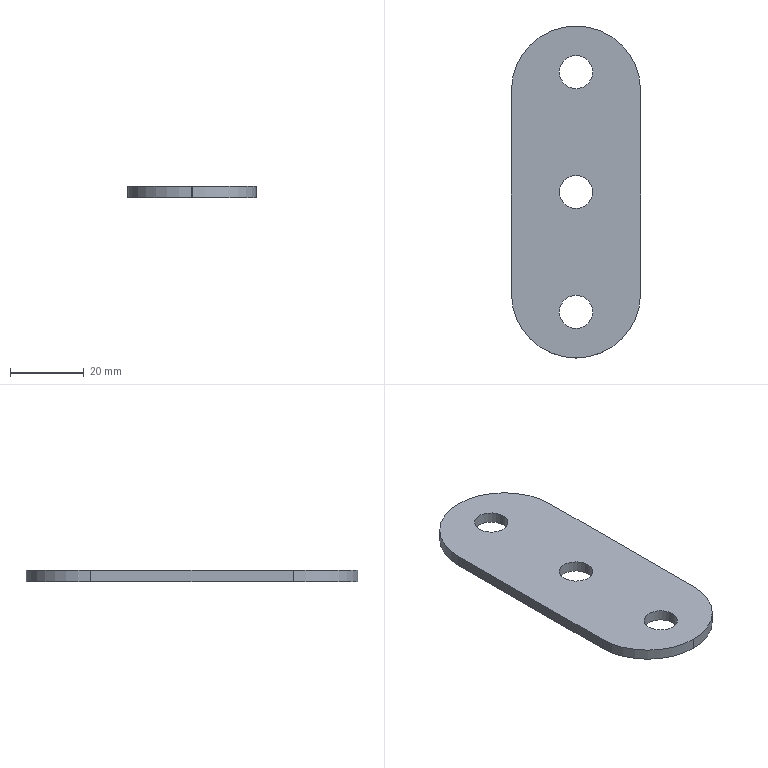Part | STEP file | 5091502 | 1 solid | 13 faces | box 35 x 90 x 3 mm | volume 8089 mm3 | cylinder 7 | plane 6 | commonest cylinder face diameters 34.998 x4 9 x3
STEP:
#1=CARTESIAN_POINT('',(0.,0.,0.));
#2=DIRECTION('',(0.,0.,1.));
#3=DIRECTION('',(1.,0.,0.));
#4=AXIS2_PLACEMENT_3D('',#1,#2,#3);
#5=CARTESIAN_POINT('',(4.5,0.,3.));
#6=VERTEX_POINT('',#5);
#7=CARTESIAN_POINT('',(0.,0.,3.));
#8=DIRECTION('',(0.,0.,1.));
#9=DIRECTION('',(1.,0.,0.));
#10=AXIS2_PLACEMENT_3D('',#7,#8,#9);
#11=CIRCLE('',#10,4.5);
#12=CARTESIAN_POINT('',(0.001,27.501,3.));
#13=DIRECTION('',(0.,0.,-1.));
#14=DIRECTION('',(-1.,0.,0.));
#15=AXIS2_PLACEMENT_3D('',#12,#13,#14);
#16=PLANE('',#15);
#17=CARTESIAN_POINT('',(-4.499,-27.501));
#18=CARTESIAN_POINT('',(-4.499,-19.707));
#19=CARTESIAN_POINT('',(2.251,-23.604));
#20=CARTESIAN_POINT('',(9.001,-27.501));
#21=CARTESIAN_POINT('',(2.251,-31.398));
#22=CARTESIAN_POINT('',(-4.499,-35.295));
#23=CARTESIAN_POINT('',(-4.499,-27.501));
#24=(BOUNDED_CURVE()B_SPLINE_CURVE(2,(#17,#18,#19,#20,#21,#22,#23),.UNSPECIFIED.,.T.,.F.)B_SPLINE_CURVE_WITH_KNOTS((1,2,2,2,2,1),(-2.094,0.,2.094,4.189,6.283,8.378),.UNSPECIFIED.)CURVE()GEOMETRIC_REPRESENTATION_ITEM()RATIONAL_B_SPLINE_CURVE((1.,0.5,1.,0.5,1.,0.5,1.))REPRESENTATION_ITEM(''));
#25=(GEOMETRIC_REPRESENTATION_CONTEXT(2)PARAMETRIC_REPRESENTATION_CONTEXT()REPRESENTATION_CONTEXT('',''));
#26=DEFINITIONAL_REPRESENTATION('',(#24),#25);
#27=PCURVE('',#16,#26);
#28=CARTESIAN_POINT('',(0.,0.,3.));
#29=DIRECTION('',(0.,0.,-1.));
#30=DIRECTION('',(-1.,0.,0.));
#31=AXIS2_PLACEMENT_3D('',#28,#29,#30);
#32=CYLINDRICAL_SURFACE('',#31,4.5);
#33=CARTESIAN_POINT('',(9.425,0.));
#34=DIRECTION('',(-1.,0.));
#35=VECTOR('',#34,1.);
#36=LINE('',#33,#35);
#37=(GEOMETRIC_REPRESENTATION_CONTEXT(2)PARAMETRIC_REPRESENTATION_CONTEXT()REPRESENTATION_CONTEXT('',''));
#38=DEFINITIONAL_REPRESENTATION('',(#36),#37);
#39=PCURVE('',#32,#38);
#40=SURFACE_CURVE('',#11,(#27,#39),.PCURVE_S1.);
#41=EDGE_CURVE('',#6,#6,#40,.T.);
#42=ORIENTED_EDGE('',*,*,#41,.F.);
#43=EDGE_LOOP('',(#42));
#44=FACE_BOUND('',#43,.T.);
#45=CARTESIAN_POINT('',(17.5,27.501,3.));
#46=VERTEX_POINT('',#45);
#47=CARTESIAN_POINT('',(0.001,45.,3.));
#48=VERTEX_POINT('',#47);
#49=CARTESIAN_POINT('',(0.001,27.501,3.));
#50=DIRECTION('',(0.,0.,1.));
#51=DIRECTION('',(-1.,0.,0.));
#52=AXIS2_PLACEMENT_3D('',#49,#50,#51);
#53=CIRCLE('',#52,17.499);
#54=CARTESIAN_POINT('',(17.499,0.));
#55=CARTESIAN_POINT('',(17.499,-30.309));
#56=CARTESIAN_POINT('',(-8.749,-15.155));
#57=CARTESIAN_POINT('',(-34.998,0.));
#58=CARTESIAN_POINT('',(-8.749,15.155));
#59=CARTESIAN_POINT('',(17.499,30.309));
#60=CARTESIAN_POINT('',(17.499,0.));
#61=(BOUNDED_CURVE()B_SPLINE_CURVE(2,(#54,#55,#56,#57,#58,#59,#60),.UNSPECIFIED.,.T.,.F.)B_SPLINE_CURVE_WITH_KNOTS((1,2,2,2,2,1),(-2.094,0.,2.094,4.189,6.283,8.378),.UNSPECIFIED.)CURVE()GEOMETRIC_REPRESENTATION_ITEM()RATIONAL_B_SPLINE_CURVE((1.,0.5,1.,0.5,1.,0.5,1.))REPRESENTATION_ITEM(''));
#62=(GEOMETRIC_REPRESENTATION_CONTEXT(2)PARAMETRIC_REPRESENTATION_CONTEXT()REPRESENTATION_CONTEXT('',''));
#63=DEFINITIONAL_REPRESENTATION('',(#61),#62);
#64=PCURVE('',#16,#63);
#65=CARTESIAN_POINT('',(0.001,27.501,3.));
#66=DIRECTION('',(0.,0.,-1.));
#67=DIRECTION('',(-1.,0.,0.));
#68=AXIS2_PLACEMENT_3D('',#65,#66,#67);
#69=CYLINDRICAL_SURFACE('',#68,17.499);
#70=CARTESIAN_POINT('',(6.283,0.));
#71=DIRECTION('',(-1.,0.));
#72=VECTOR('',#71,1.);
#73=LINE('',#70,#72);
#74=(GEOMETRIC_REPRESENTATION_CONTEXT(2)PARAMETRIC_REPRESENTATION_CONTEXT()REPRESENTATION_CONTEXT('',''));
#75=DEFINITIONAL_REPRESENTATION('',(#73),#74);
#76=PCURVE('',#69,#75);
#77=SURFACE_CURVE('',#53,(#64,#76),.PCURVE_S1.);
#78=EDGE_CURVE('',#46,#48,#77,.T.);
#79=ORIENTED_EDGE('',*,*,#78,.T.);
#80=CARTESIAN_POINT('',(-0.001,45.,3.));
#81=VERTEX_POINT('',#80);
#82=CARTESIAN_POINT('',(-0.001,45.,3.));
#83=DIRECTION('',(-1.,0.,0.));
#84=VECTOR('',#83,1.);
#85=LINE('',#82,#84);
#86=CARTESIAN_POINT('',(0.002,17.499));
#87=DIRECTION('',(1.,0.));
#88=VECTOR('',#87,1.);
#89=LINE('',#86,#88);
#90=(GEOMETRIC_REPRESENTATION_CONTEXT(2)PARAMETRIC_REPRESENTATION_CONTEXT()REPRESENTATION_CONTEXT('',''));
#91=DEFINITIONAL_REPRESENTATION('',(#89),#90);
#92=PCURVE('',#16,#91);
#93=CARTESIAN_POINT('',(-0.001,45.,3.));
#94=DIRECTION('',(0.,-1.,0.));
#95=DIRECTION('',(0.,0.,-1.));
#96=AXIS2_PLACEMENT_3D('',#93,#94,#95);
#97=PLANE('',#96);
#98=CARTESIAN_POINT('',(0.,0.));
#99=DIRECTION('',(0.,-1.));
#100=VECTOR('',#99,1.);
#101=LINE('',#98,#100);
#102=(GEOMETRIC_REPRESENTATION_CONTEXT(2)PARAMETRIC_REPRESENTATION_CONTEXT()REPRESENTATION_CONTEXT('',''));
#103=DEFINITIONAL_REPRESENTATION('',(#101),#102);
#104=PCURVE('',#97,#103);
#105=SURFACE_CURVE('',#85,(#92,#104),.PCURVE_S1.);
#106=EDGE_CURVE('',#48,#81,#105,.T.);
#107=ORIENTED_EDGE('',*,*,#106,.T.);
#108=CARTESIAN_POINT('',(-17.5,27.501,3.));
#109=VERTEX_POINT('',#108);
#110=CARTESIAN_POINT('',(-0.001,27.501,3.));
#111=DIRECTION('',(0.,0.,1.));
#112=DIRECTION('',(-1.,0.,0.));
#113=AXIS2_PLACEMENT_3D('',#110,#111,#112);
#114=CIRCLE('',#113,17.499);
#115=CARTESIAN_POINT('',(17.501,0.));
#116=CARTESIAN_POINT('',(17.501,-30.309));
#117=CARTESIAN_POINT('',(-8.748,-15.155));
#118=CARTESIAN_POINT('',(-34.996,0.));
#119=CARTESIAN_POINT('',(-8.748,15.155));
#120=CARTESIAN_POINT('',(17.501,30.309));
#121=CARTESIAN_POINT('',(17.501,0.));
#122=(BOUNDED_CURVE()B_SPLINE_CURVE(2,(#115,#116,#117,#118,#119,#120,#121),.UNSPECIFIED.,.T.,.F.)B_SPLINE_CURVE_WITH_KNOTS((1,2,2,2,2,1),(-2.094,0.,2.094,4.189,6.283,8.378),.UNSPECIFIED.)CURVE()GEOMETRIC_REPRESENTATION_ITEM()RATIONAL_B_SPLINE_CURVE((1.,0.5,1.,0.5,1.,0.5,1.))REPRESENTATION_ITEM(''));
#123=(GEOMETRIC_REPRESENTATION_CONTEXT(2)PARAMETRIC_REPRESENTATION_CONTEXT()REPRESENTATION_CONTEXT('',''));
#124=DEFINITIONAL_REPRESENTATION('',(#122),#123);
#125=PCURVE('',#16,#124);
#126=CARTESIAN_POINT('',(-0.001,27.501,3.));
#127=DIRECTION('',(0.,0.,-1.));
#128=DIRECTION('',(-1.,0.,0.));
#129=AXIS2_PLACEMENT_3D('',#126,#127,#128);
#130=CYLINDRICAL_SURFACE('',#129,17.499);
#131=CARTESIAN_POINT('',(6.283,0.));
#132=DIRECTION('',(-1.,0.));
#133=VECTOR('',#132,1.);
#134=LINE('',#131,#133);
#135=(GEOMETRIC_REPRESENTATION_CONTEXT(2)PARAMETRIC_REPRESENTATION_CONTEXT()REPRESENTATION_CONTEXT('',''));
#136=DEFINITIONAL_REPRESENTATION('',(#134),#135);
#137=PCURVE('',#130,#136);
#138=SURFACE_CURVE('',#114,(#125,#137),.PCURVE_S1.);
#139=EDGE_CURVE('',#81,#109,#138,.T.);
#140=ORIENTED_EDGE('',*,*,#139,.T.);
#141=CARTESIAN_POINT('',(-17.5,-27.501,3.));
#142=VERTEX_POINT('',#141);
#143=CARTESIAN_POINT('',(-17.5,27.501,3.));
#144=DIRECTION('',(0.,-1.,0.));
#145=VECTOR('',#144,1.);
#146=LINE('',#143,#145);
#147=CARTESIAN_POINT('',(17.501,0.));
#148=DIRECTION('',(0.,-1.));
#149=VECTOR('',#148,1.);
#150=LINE('',#147,#149);
#151=(GEOMETRIC_REPRESENTATION_CONTEXT(2)PARAMETRIC_REPRESENTATION_CONTEXT()REPRESENTATION_CONTEXT('',''));
#152=DEFINITIONAL_REPRESENTATION('',(#150),#151);
#153=PCURVE('',#16,#152);
#154=CARTESIAN_POINT('',(-17.5,27.501,3.));
#155=DIRECTION('',(1.,0.,0.));
#156=DIRECTION('',(0.,1.,0.));
#157=AXIS2_PLACEMENT_3D('',#154,#155,#156);
#158=PLANE('',#157);
#159=CARTESIAN_POINT('',(0.,0.));
#160=DIRECTION('',(-1.,0.));
#161=VECTOR('',#160,1.);
#162=LINE('',#159,#161);
#163=(GEOMETRIC_REPRESENTATION_CONTEXT(2)PARAMETRIC_REPRESENTATION_CONTEXT()REPRESENTATION_CONTEXT('',''));
#164=DEFINITIONAL_REPRESENTATION('',(#162),#163);
#165=PCURVE('',#158,#164);
#166=SURFACE_CURVE('',#146,(#153,#165),.PCURVE_S1.);
#167=EDGE_CURVE('',#109,#142,#166,.T.);
#168=ORIENTED_EDGE('',*,*,#167,.T.);
#169=CARTESIAN_POINT('',(-0.001,-45.,3.));
#170=VERTEX_POINT('',#169);
#171=CARTESIAN_POINT('',(-0.001,-27.501,3.));
#172=DIRECTION('',(0.,0.,1.));
#173=DIRECTION('',(-1.,0.,0.));
#174=AXIS2_PLACEMENT_3D('',#171,#172,#173);
#175=CIRCLE('',#174,17.499);
#176=CARTESIAN_POINT('',(17.501,-55.002));
#177=CARTESIAN_POINT('',(17.501,-85.311));
#178=CARTESIAN_POINT('',(-8.748,-70.157));
#179=CARTESIAN_POINT('',(-34.996,-55.002));
#180=CARTESIAN_POINT('',(-8.748,-39.847));
#181=CARTESIAN_POINT('',(17.501,-24.693));
#182=CARTESIAN_POINT('',(17.501,-55.002));
#183=(BOUNDED_CURVE()B_SPLINE_CURVE(2,(#176,#177,#178,#179,#180,#181,#182),.UNSPECIFIED.,.T.,.F.)B_SPLINE_CURVE_WITH_KNOTS((1,2,2,2,2,1),(-2.094,0.,2.094,4.189,6.283,8.378),.UNSPECIFIED.)CURVE()GEOMETRIC_REPRESENTATION_ITEM()RATIONAL_B_SPLINE_CURVE((1.,0.5,1.,0.5,1.,0.5,1.))REPRESENTATION_ITEM(''));
#184=(GEOMETRIC_REPRESENTATION_CONTEXT(2)PARAMETRIC_REPRESENTATION_CONTEXT()REPRESENTATION_CONTEXT('',''));
#185=DEFINITIONAL_REPRESENTATION('',(#183),#184);
#186=PCURVE('',#16,#185);
#187=CARTESIAN_POINT('',(-0.001,-27.501,3.));
#188=DIRECTION('',(0.,0.,-1.));
#189=DIRECTION('',(-1.,0.,0.));
#190=AXIS2_PLACEMENT_3D('',#187,#188,#189);
#191=CYLINDRICAL_SURFACE('',#190,17.499);
#192=CARTESIAN_POINT('',(6.283,0.));
#193=DIRECTION('',(-1.,0.));
#194=VECTOR('',#193,1.);
#195=LINE('',#192,#194);
#196=(GEOMETRIC_REPRESENTATION_CONTEXT(2)PARAMETRIC_REPRESENTATION_CONTEXT()REPRESENTATION_CONTEXT('',''));
#197=DEFINITIONAL_REPRESENTATION('',(#195),#196);
#198=PCURVE('',#191,#197);
#199=SURFACE_CURVE('',#175,(#186,#198),.PCURVE_S1.);
#200=EDGE_CURVE('',#142,#170,#199,.T.);
#201=ORIENTED_EDGE('',*,*,#200,.T.);
#202=CARTESIAN_POINT('',(0.001,-45.,3.));
#203=VERTEX_POINT('',#202);
#204=CARTESIAN_POINT('',(-0.001,-45.,3.));
#205=DIRECTION('',(1.,0.,0.));
#206=VECTOR('',#205,1.);
#207=LINE('',#204,#206);
#208=CARTESIAN_POINT('',(0.002,-72.501));
#209=DIRECTION('',(-1.,0.));
#210=VECTOR('',#209,1.);
#211=LINE('',#208,#210);
#212=(GEOMETRIC_REPRESENTATION_CONTEXT(2)PARAMETRIC_REPRESENTATION_CONTEXT()REPRESENTATION_CONTEXT('',''));
#213=DEFINITIONAL_REPRESENTATION('',(#211),#212);
#214=PCURVE('',#16,#213);
#215=CARTESIAN_POINT('',(-0.001,-45.,3.));
#216=DIRECTION('',(0.,1.,0.));
#217=DIRECTION('',(0.,0.,1.));
#218=AXIS2_PLACEMENT_3D('',#215,#216,#217);
#219=PLANE('',#218);
#220=CARTESIAN_POINT('',(0.,0.));
#221=DIRECTION('',(0.,1.));
#222=VECTOR('',#221,1.);
#223=LINE('',#220,#222);
#224=(GEOMETRIC_REPRESENTATION_CONTEXT(2)PARAMETRIC_REPRESENTATION_CONTEXT()REPRESENTATION_CONTEXT('',''));
#225=DEFINITIONAL_REPRESENTATION('',(#223),#224);
#226=PCURVE('',#219,#225);
#227=SURFACE_CURVE('',#207,(#214,#226),.PCURVE_S1.);
#228=EDGE_CURVE('',#170,#203,#227,.T.);
#229=ORIENTED_EDGE('',*,*,#228,.T.);
#230=CARTESIAN_POINT('',(17.5,-27.501,3.));
#231=VERTEX_POINT('',#230);
#232=CARTESIAN_POINT('',(0.001,-27.501,3.));
#233=DIRECTION('',(0.,0.,1.));
#234=DIRECTION('',(-1.,0.,0.));
#235=AXIS2_PLACEMENT_3D('',#232,#233,#234);
#236=CIRCLE('',#235,17.499);
#237=CARTESIAN_POINT('',(17.499,-55.002));
#238=CARTESIAN_POINT('',(17.499,-85.311));
#239=CARTESIAN_POINT('',(-8.749,-70.157));
#240=CARTESIAN_POINT('',(-34.998,-55.002));
#241=CARTESIAN_POINT('',(-8.749,-39.847));
#242=CARTESIAN_POINT('',(17.499,-24.693));
#243=CARTESIAN_POINT('',(17.499,-55.002));
#244=(BOUNDED_CURVE()B_SPLINE_CURVE(2,(#237,#238,#239,#240,#241,#242,#243),.UNSPECIFIED.,.T.,.F.)B_SPLINE_CURVE_WITH_KNOTS((1,2,2,2,2,1),(-2.094,0.,2.094,4.189,6.283,8.378),.UNSPECIFIED.)CURVE()GEOMETRIC_REPRESENTATION_ITEM()RATIONAL_B_SPLINE_CURVE((1.,0.5,1.,0.5,1.,0.5,1.))REPRESENTATION_ITEM(''));
#245=(GEOMETRIC_REPRESENTATION_CONTEXT(2)PARAMETRIC_REPRESENTATION_CONTEXT()REPRESENTATION_CONTEXT('',''));
#246=DEFINITIONAL_REPRESENTATION('',(#244),#245);
#247=PCURVE('',#16,#246);
#248=CARTESIAN_POINT('',(0.001,-27.501,3.));
#249=DIRECTION('',(0.,0.,-1.));
#250=DIRECTION('',(-1.,0.,0.));
#251=AXIS2_PLACEMENT_3D('',#248,#249,#250);
#252=CYLINDRICAL_SURFACE('',#251,17.499);
#253=CARTESIAN_POINT('',(6.283,0.));
#254=DIRECTION('',(-1.,0.));
#255=VECTOR('',#254,1.);
#256=LINE('',#253,#255);
#257=(GEOMETRIC_REPRESENTATION_CONTEXT(2)PARAMETRIC_REPRESENTATION_CONTEXT()REPRESENTATION_CONTEXT('',''));
#258=DEFINITIONAL_REPRESENTATION('',(#256),#257);
#259=PCURVE('',#252,#258);
#260=SURFACE_CURVE('',#236,(#247,#259),.PCURVE_S1.);
#261=EDGE_CURVE('',#203,#231,#260,.T.);
#262=ORIENTED_EDGE('',*,*,#261,.T.);
#263=CARTESIAN_POINT('',(17.5,27.501,3.));
#264=DIRECTION('',(0.,1.,0.));
#265=VECTOR('',#264,1.);
#266=LINE('',#263,#265);
#267=CARTESIAN_POINT('',(-17.499,0.));
#268=DIRECTION('',(0.,1.));
#269=VECTOR('',#268,1.);
#270=LINE('',#267,#269);
#271=(GEOMETRIC_REPRESENTATION_CONTEXT(2)PARAMETRIC_REPRESENTATION_CONTEXT()REPRESENTATION_CONTEXT('',''));
#272=DEFINITIONAL_REPRESENTATION('',(#270),#271);
#273=PCURVE('',#16,#272);
#274=CARTESIAN_POINT('',(17.5,27.501,3.));
#275=DIRECTION('',(-1.,0.,0.));
#276=DIRECTION('',(0.,0.,1.));
#277=AXIS2_PLACEMENT_3D('',#274,#275,#276);
#278=PLANE('',#277);
#279=CARTESIAN_POINT('',(0.,0.));
#280=DIRECTION('',(0.,1.));
#281=VECTOR('',#280,1.);
#282=LINE('',#279,#281);
#283=(GEOMETRIC_REPRESENTATION_CONTEXT(2)PARAMETRIC_REPRESENTATION_CONTEXT()REPRESENTATION_CONTEXT('',''));
#284=DEFINITIONAL_REPRESENTATION('',(#282),#283);
#285=PCURVE('',#278,#284);
#286=SURFACE_CURVE('',#266,(#273,#285),.PCURVE_S1.);
#287=EDGE_CURVE('',#231,#46,#286,.T.);
#288=ORIENTED_EDGE('',*,*,#287,.T.);
#289=EDGE_LOOP('',(#79,#107,#140,#168,#201,#229,#262,#288));
#290=FACE_BOUND('',#289,.T.);
#291=CARTESIAN_POINT('',(4.5,32.5,3.));
#292=VERTEX_POINT('',#291);
#293=CARTESIAN_POINT('',(0.,32.5,3.));
#294=DIRECTION('',(0.,0.,1.));
#295=DIRECTION('',(1.,0.,0.));
#296=AXIS2_PLACEMENT_3D('',#293,#294,#295);
#297=CIRCLE('',#296,4.5);
#298=CARTESIAN_POINT('',(-4.499,4.999));
#299=CARTESIAN_POINT('',(-4.499,12.793));
#300=CARTESIAN_POINT('',(2.251,8.896));
#301=CARTESIAN_POINT('',(9.001,4.999));
#302=CARTESIAN_POINT('',(2.251,1.102));
#303=CARTESIAN_POINT('',(-4.499,-2.795));
#304=CARTESIAN_POINT('',(-4.499,4.999));
#305=(BOUNDED_CURVE()B_SPLINE_CURVE(2,(#298,#299,#300,#301,#302,#303,#304),.UNSPECIFIED.,.T.,.F.)B_SPLINE_CURVE_WITH_KNOTS((1,2,2,2,2,1),(-2.094,0.,2.094,4.189,6.283,8.378),.UNSPECIFIED.)CURVE()GEOMETRIC_REPRESENTATION_ITEM()RATIONAL_B_SPLINE_CURVE((1.,0.5,1.,0.5,1.,0.5,1.))REPRESENTATION_ITEM(''));
#306=(GEOMETRIC_REPRESENTATION_CONTEXT(2)PARAMETRIC_REPRESENTATION_CONTEXT()REPRESENTATION_CONTEXT('',''));
#307=DEFINITIONAL_REPRESENTATION('',(#305),#306);
#308=PCURVE('',#16,#307);
#309=CARTESIAN_POINT('',(0.,32.5,3.));
#310=DIRECTION('',(0.,0.,-1.));
#311=DIRECTION('',(-1.,0.,0.));
#312=AXIS2_PLACEMENT_3D('',#309,#310,#311);
#313=CYLINDRICAL_SURFACE('',#312,4.5);
#314=CARTESIAN_POINT('',(9.425,0.));
#315=DIRECTION('',(-1.,0.));
#316=VECTOR('',#315,1.);
#317=LINE('',#314,#316);
#318=(GEOMETRIC_REPRESENTATION_CONTEXT(2)PARAMETRIC_REPRESENTATION_CONTEXT()REPRESENTATION_CONTEXT('',''));
#319=DEFINITIONAL_REPRESENTATION('',(#317),#318);
#320=PCURVE('',#313,#319);
#321=SURFACE_CURVE('',#297,(#308,#320),.PCURVE_S1.);
#322=EDGE_CURVE('',#292,#292,#321,.T.);
#323=ORIENTED_EDGE('',*,*,#322,.F.);
#324=EDGE_LOOP('',(#323));
#325=FACE_BOUND('',#324,.T.);
#326=CARTESIAN_POINT('',(4.5,-32.5,3.));
#327=VERTEX_POINT('',#326);
#328=CARTESIAN_POINT('',(0.,-32.5,3.));
#329=DIRECTION('',(0.,0.,1.));
#330=DIRECTION('',(1.,0.,0.));
#331=AXIS2_PLACEMENT_3D('',#328,#329,#330);
#332=CIRCLE('',#331,4.5);
#333=CARTESIAN_POINT('',(-4.499,-60.001));
#334=CARTESIAN_POINT('',(-4.499,-52.207));
#335=CARTESIAN_POINT('',(2.251,-56.104));
#336=CARTESIAN_POINT('',(9.001,-60.001));
#337=CARTESIAN_POINT('',(2.251,-63.898));
#338=CARTESIAN_POINT('',(-4.499,-67.795));
#339=CARTESIAN_POINT('',(-4.499,-60.001));
#340=(BOUNDED_CURVE()B_SPLINE_CURVE(2,(#333,#334,#335,#336,#337,#338,#339),.UNSPECIFIED.,.T.,.F.)B_SPLINE_CURVE_WITH_KNOTS((1,2,2,2,2,1),(-2.094,0.,2.094,4.189,6.283,8.378),.UNSPECIFIED.)CURVE()GEOMETRIC_REPRESENTATION_ITEM()RATIONAL_B_SPLINE_CURVE((1.,0.5,1.,0.5,1.,0.5,1.))REPRESENTATION_ITEM(''));
#341=(GEOMETRIC_REPRESENTATION_CONTEXT(2)PARAMETRIC_REPRESENTATION_CONTEXT()REPRESENTATION_CONTEXT('',''));
#342=DEFINITIONAL_REPRESENTATION('',(#340),#341);
#343=PCURVE('',#16,#342);
#344=CARTESIAN_POINT('',(0.,-32.5,3.));
#345=DIRECTION('',(0.,0.,-1.));
#346=DIRECTION('',(-1.,0.,0.));
#347=AXIS2_PLACEMENT_3D('',#344,#345,#346);
#348=CYLINDRICAL_SURFACE('',#347,4.5);
#349=CARTESIAN_POINT('',(9.425,0.));
#350=DIRECTION('',(-1.,0.));
#351=VECTOR('',#350,1.);
#352=LINE('',#349,#351);
#353=(GEOMETRIC_REPRESENTATION_CONTEXT(2)PARAMETRIC_REPRESENTATION_CONTEXT()REPRESENTATION_CONTEXT('',''));
#354=DEFINITIONAL_REPRESENTATION('',(#352),#353);
#355=PCURVE('',#348,#354);
#356=SURFACE_CURVE('',#332,(#343,#355),.PCURVE_S1.);
#357=EDGE_CURVE('',#327,#327,#356,.T.);
#358=ORIENTED_EDGE('',*,*,#357,.F.);
#359=EDGE_LOOP('',(#358));
#360=FACE_BOUND('',#359,.T.);
#361=ADVANCED_FACE('',(#44,#290,#325,#360),#16,.F.);
#362=CARTESIAN_POINT('',(4.5,0.,0.));
#363=VERTEX_POINT('',#362);
#364=CARTESIAN_POINT('',(0.,0.,0.));
#365=DIRECTION('',(0.,0.,1.));
#366=DIRECTION('',(1.,0.,0.));
#367=AXIS2_PLACEMENT_3D('',#364,#365,#366);
#368=CIRCLE('',#367,4.5);
#369=CARTESIAN_POINT('',(0.001,27.501,0.));
#370=DIRECTION('',(0.,0.,-1.));
#371=DIRECTION('',(-1.,0.,0.));
#372=AXIS2_PLACEMENT_3D('',#369,#370,#371);
#373=PLANE('',#372);
#374=CARTESIAN_POINT('',(-4.499,-27.501));
#375=CARTESIAN_POINT('',(-4.499,-19.707));
#376=CARTESIAN_POINT('',(2.251,-23.604));
#377=CARTESIAN_POINT('',(9.001,-27.501));
#378=CARTESIAN_POINT('',(2.251,-31.398));
#379=CARTESIAN_POINT('',(-4.499,-35.295));
#380=CARTESIAN_POINT('',(-4.499,-27.501));
#381=(BOUNDED_CURVE()B_SPLINE_CURVE(2,(#374,#375,#376,#377,#378,#379,#380),.UNSPECIFIED.,.T.,.F.)B_SPLINE_CURVE_WITH_KNOTS((1,2,2,2,2,1),(-2.094,0.,2.094,4.189,6.283,8.378),.UNSPECIFIED.)CURVE()GEOMETRIC_REPRESENTATION_ITEM()RATIONAL_B_SPLINE_CURVE((1.,0.5,1.,0.5,1.,0.5,1.))REPRESENTATION_ITEM(''));
#382=(GEOMETRIC_REPRESENTATION_CONTEXT(2)PARAMETRIC_REPRESENTATION_CONTEXT()REPRESENTATION_CONTEXT('',''));
#383=DEFINITIONAL_REPRESENTATION('',(#381),#382);
#384=PCURVE('',#373,#383);
#385=CARTESIAN_POINT('',(9.425,3.));
#386=DIRECTION('',(-1.,0.));
#387=VECTOR('',#386,1.);
#388=LINE('',#385,#387);
#389=(GEOMETRIC_REPRESENTATION_CONTEXT(2)PARAMETRIC_REPRESENTATION_CONTEXT()REPRESENTATION_CONTEXT('',''));
#390=DEFINITIONAL_REPRESENTATION('',(#388),#389);
#391=PCURVE('',#32,#390);
#392=SURFACE_CURVE('',#368,(#384,#391),.PCURVE_S1.);
#393=EDGE_CURVE('',#363,#363,#392,.T.);
#394=ORIENTED_EDGE('',*,*,#393,.T.);
#395=EDGE_LOOP('',(#394));
#396=FACE_BOUND('',#395,.T.);
#397=CARTESIAN_POINT('',(17.5,27.501,0.));
#398=VERTEX_POINT('',#397);
#399=CARTESIAN_POINT('',(0.001,45.,0.));
#400=VERTEX_POINT('',#399);
#401=CARTESIAN_POINT('',(0.001,27.501,0.));
#402=DIRECTION('',(0.,0.,1.));
#403=DIRECTION('',(-1.,0.,0.));
#404=AXIS2_PLACEMENT_3D('',#401,#402,#403);
#405=CIRCLE('',#404,17.499);
#406=CARTESIAN_POINT('',(17.499,0.));
#407=CARTESIAN_POINT('',(17.499,-30.309));
#408=CARTESIAN_POINT('',(-8.749,-15.155));
#409=CARTESIAN_POINT('',(-34.998,0.));
#410=CARTESIAN_POINT('',(-8.749,15.155));
#411=CARTESIAN_POINT('',(17.499,30.309));
#412=CARTESIAN_POINT('',(17.499,0.));
#413=(BOUNDED_CURVE()B_SPLINE_CURVE(2,(#406,#407,#408,#409,#410,#411,#412),.UNSPECIFIED.,.T.,.F.)B_SPLINE_CURVE_WITH_KNOTS((1,2,2,2,2,1),(-2.094,0.,2.094,4.189,6.283,8.378),.UNSPECIFIED.)CURVE()GEOMETRIC_REPRESENTATION_ITEM()RATIONAL_B_SPLINE_CURVE((1.,0.5,1.,0.5,1.,0.5,1.))REPRESENTATION_ITEM(''));
#414=(GEOMETRIC_REPRESENTATION_CONTEXT(2)PARAMETRIC_REPRESENTATION_CONTEXT()REPRESENTATION_CONTEXT('',''));
#415=DEFINITIONAL_REPRESENTATION('',(#413),#414);
#416=PCURVE('',#373,#415);
#417=CARTESIAN_POINT('',(6.283,3.));
#418=DIRECTION('',(-1.,0.));
#419=VECTOR('',#418,1.);
#420=LINE('',#417,#419);
#421=(GEOMETRIC_REPRESENTATION_CONTEXT(2)PARAMETRIC_REPRESENTATION_CONTEXT()REPRESENTATION_CONTEXT('',''));
#422=DEFINITIONAL_REPRESENTATION('',(#420),#421);
#423=PCURVE('',#69,#422);
#424=SURFACE_CURVE('',#405,(#416,#423),.PCURVE_S1.);
#425=EDGE_CURVE('',#398,#400,#424,.T.);
#426=ORIENTED_EDGE('',*,*,#425,.F.);
#427=CARTESIAN_POINT('',(17.5,-27.501,0.));
#428=VERTEX_POINT('',#427);
#429=CARTESIAN_POINT('',(17.5,27.501,0.));
#430=DIRECTION('',(0.,1.,0.));
#431=VECTOR('',#430,1.);
#432=LINE('',#429,#431);
#433=CARTESIAN_POINT('',(-17.499,0.));
#434=DIRECTION('',(0.,1.));
#435=VECTOR('',#434,1.);
#436=LINE('',#433,#435);
#437=(GEOMETRIC_REPRESENTATION_CONTEXT(2)PARAMETRIC_REPRESENTATION_CONTEXT()REPRESENTATION_CONTEXT('',''));
#438=DEFINITIONAL_REPRESENTATION('',(#436),#437);
#439=PCURVE('',#373,#438);
#440=CARTESIAN_POINT('',(-3.,0.));
#441=DIRECTION('',(0.,1.));
#442=VECTOR('',#441,1.);
#443=LINE('',#440,#442);
#444=(GEOMETRIC_REPRESENTATION_CONTEXT(2)PARAMETRIC_REPRESENTATION_CONTEXT()REPRESENTATION_CONTEXT('',''));
#445=DEFINITIONAL_REPRESENTATION('',(#443),#444);
#446=PCURVE('',#278,#445);
#447=SURFACE_CURVE('',#432,(#439,#446),.PCURVE_S1.);
#448=EDGE_CURVE('',#428,#398,#447,.T.);
#449=ORIENTED_EDGE('',*,*,#448,.F.);
#450=CARTESIAN_POINT('',(0.001,-45.,0.));
#451=VERTEX_POINT('',#450);
#452=CARTESIAN_POINT('',(0.001,-27.501,0.));
#453=DIRECTION('',(0.,0.,1.));
#454=DIRECTION('',(-1.,0.,0.));
#455=AXIS2_PLACEMENT_3D('',#452,#453,#454);
#456=CIRCLE('',#455,17.499);
#457=CARTESIAN_POINT('',(17.499,-55.002));
#458=CARTESIAN_POINT('',(17.499,-85.311));
#459=CARTESIAN_POINT('',(-8.749,-70.157));
#460=CARTESIAN_POINT('',(-34.998,-55.002));
#461=CARTESIAN_POINT('',(-8.749,-39.847));
#462=CARTESIAN_POINT('',(17.499,-24.693));
#463=CARTESIAN_POINT('',(17.499,-55.002));
#464=(BOUNDED_CURVE()B_SPLINE_CURVE(2,(#457,#458,#459,#460,#461,#462,#463),.UNSPECIFIED.,.T.,.F.)B_SPLINE_CURVE_WITH_KNOTS((1,2,2,2,2,1),(-2.094,0.,2.094,4.189,6.283,8.378),.UNSPECIFIED.)CURVE()GEOMETRIC_REPRESENTATION_ITEM()RATIONAL_B_SPLINE_CURVE((1.,0.5,1.,0.5,1.,0.5,1.))REPRESENTATION_ITEM(''));
#465=(GEOMETRIC_REPRESENTATION_CONTEXT(2)PARAMETRIC_REPRESENTATION_CONTEXT()REPRESENTATION_CONTEXT('',''));
#466=DEFINITIONAL_REPRESENTATION('',(#464),#465);
#467=PCURVE('',#373,#466);
#468=CARTESIAN_POINT('',(6.283,3.));
#469=DIRECTION('',(-1.,0.));
#470=VECTOR('',#469,1.);
#471=LINE('',#468,#470);
#472=(GEOMETRIC_REPRESENTATION_CONTEXT(2)PARAMETRIC_REPRESENTATION_CONTEXT()REPRESENTATION_CONTEXT('',''));
#473=DEFINITIONAL_REPRESENTATION('',(#471),#472);
#474=PCURVE('',#252,#473);
#475=SURFACE_CURVE('',#456,(#467,#474),.PCURVE_S1.);
#476=EDGE_CURVE('',#451,#428,#475,.T.);
#477=ORIENTED_EDGE('',*,*,#476,.F.);
#478=CARTESIAN_POINT('',(-0.001,-45.,0.));
#479=VERTEX_POINT('',#478);
#480=CARTESIAN_POINT('',(-0.001,-45.,0.));
#481=DIRECTION('',(1.,0.,0.));
#482=VECTOR('',#481,1.);
#483=LINE('',#480,#482);
#484=CARTESIAN_POINT('',(0.002,-72.501));
#485=DIRECTION('',(-1.,0.));
#486=VECTOR('',#485,1.);
#487=LINE('',#484,#486);
#488=(GEOMETRIC_REPRESENTATION_CONTEXT(2)PARAMETRIC_REPRESENTATION_CONTEXT()REPRESENTATION_CONTEXT('',''));
#489=DEFINITIONAL_REPRESENTATION('',(#487),#488);
#490=PCURVE('',#373,#489);
#491=CARTESIAN_POINT('',(-3.,0.));
#492=DIRECTION('',(0.,1.));
#493=VECTOR('',#492,1.);
#494=LINE('',#491,#493);
#495=(GEOMETRIC_REPRESENTATION_CONTEXT(2)PARAMETRIC_REPRESENTATION_CONTEXT()REPRESENTATION_CONTEXT('',''));
#496=DEFINITIONAL_REPRESENTATION('',(#494),#495);
#497=PCURVE('',#219,#496);
#498=SURFACE_CURVE('',#483,(#490,#497),.PCURVE_S1.);
#499=EDGE_CURVE('',#479,#451,#498,.T.);
#500=ORIENTED_EDGE('',*,*,#499,.F.);
#501=CARTESIAN_POINT('',(-17.5,-27.501,0.));
#502=VERTEX_POINT('',#501);
#503=CARTESIAN_POINT('',(-0.001,-27.501,0.));
#504=DIRECTION('',(0.,0.,1.));
#505=DIRECTION('',(-1.,0.,0.));
#506=AXIS2_PLACEMENT_3D('',#503,#504,#505);
#507=CIRCLE('',#506,17.499);
#508=CARTESIAN_POINT('',(17.501,-55.002));
#509=CARTESIAN_POINT('',(17.501,-85.311));
#510=CARTESIAN_POINT('',(-8.748,-70.157));
#511=CARTESIAN_POINT('',(-34.996,-55.002));
#512=CARTESIAN_POINT('',(-8.748,-39.847));
#513=CARTESIAN_POINT('',(17.501,-24.693));
#514=CARTESIAN_POINT('',(17.501,-55.002));
#515=(BOUNDED_CURVE()B_SPLINE_CURVE(2,(#508,#509,#510,#511,#512,#513,#514),.UNSPECIFIED.,.T.,.F.)B_SPLINE_CURVE_WITH_KNOTS((1,2,2,2,2,1),(-2.094,0.,2.094,4.189,6.283,8.378),.UNSPECIFIED.)CURVE()GEOMETRIC_REPRESENTATION_ITEM()RATIONAL_B_SPLINE_CURVE((1.,0.5,1.,0.5,1.,0.5,1.))REPRESENTATION_ITEM(''));
#516=(GEOMETRIC_REPRESENTATION_CONTEXT(2)PARAMETRIC_REPRESENTATION_CONTEXT()REPRESENTATION_CONTEXT('',''));
#517=DEFINITIONAL_REPRESENTATION('',(#515),#516);
#518=PCURVE('',#373,#517);
#519=CARTESIAN_POINT('',(6.283,3.));
#520=DIRECTION('',(-1.,0.));
#521=VECTOR('',#520,1.);
#522=LINE('',#519,#521);
#523=(GEOMETRIC_REPRESENTATION_CONTEXT(2)PARAMETRIC_REPRESENTATION_CONTEXT()REPRESENTATION_CONTEXT('',''));
#524=DEFINITIONAL_REPRESENTATION('',(#522),#523);
#525=PCURVE('',#191,#524);
#526=SURFACE_CURVE('',#507,(#518,#525),.PCURVE_S1.);
#527=EDGE_CURVE('',#502,#479,#526,.T.);
#528=ORIENTED_EDGE('',*,*,#527,.F.);
#529=CARTESIAN_POINT('',(-17.5,27.501,0.));
#530=VERTEX_POINT('',#529);
#531=CARTESIAN_POINT('',(-17.5,27.501,0.));
#532=DIRECTION('',(0.,-1.,0.));
#533=VECTOR('',#532,1.);
#534=LINE('',#531,#533);
#535=CARTESIAN_POINT('',(17.501,0.));
#536=DIRECTION('',(0.,-1.));
#537=VECTOR('',#536,1.);
#538=LINE('',#535,#537);
#539=(GEOMETRIC_REPRESENTATION_CONTEXT(2)PARAMETRIC_REPRESENTATION_CONTEXT()REPRESENTATION_CONTEXT('',''));
#540=DEFINITIONAL_REPRESENTATION('',(#538),#539);
#541=PCURVE('',#373,#540);
#542=CARTESIAN_POINT('',(0.,-3.));
#543=DIRECTION('',(-1.,0.));
#544=VECTOR('',#543,1.);
#545=LINE('',#542,#544);
#546=(GEOMETRIC_REPRESENTATION_CONTEXT(2)PARAMETRIC_REPRESENTATION_CONTEXT()REPRESENTATION_CONTEXT('',''));
#547=DEFINITIONAL_REPRESENTATION('',(#545),#546);
#548=PCURVE('',#158,#547);
#549=SURFACE_CURVE('',#534,(#541,#548),.PCURVE_S1.);
#550=EDGE_CURVE('',#530,#502,#549,.T.);
#551=ORIENTED_EDGE('',*,*,#550,.F.);
#552=CARTESIAN_POINT('',(-0.001,45.,0.));
#553=VERTEX_POINT('',#552);
#554=CARTESIAN_POINT('',(-0.001,27.501,0.));
#555=DIRECTION('',(0.,0.,1.));
#556=DIRECTION('',(-1.,0.,0.));
#557=AXIS2_PLACEMENT_3D('',#554,#555,#556);
#558=CIRCLE('',#557,17.499);
#559=CARTESIAN_POINT('',(17.501,0.));
#560=CARTESIAN_POINT('',(17.501,-30.309));
#561=CARTESIAN_POINT('',(-8.748,-15.155));
#562=CARTESIAN_POINT('',(-34.996,0.));
#563=CARTESIAN_POINT('',(-8.748,15.155));
#564=CARTESIAN_POINT('',(17.501,30.309));
#565=CARTESIAN_POINT('',(17.501,0.));
#566=(BOUNDED_CURVE()B_SPLINE_CURVE(2,(#559,#560,#561,#562,#563,#564,#565),.UNSPECIFIED.,.T.,.F.)B_SPLINE_CURVE_WITH_KNOTS((1,2,2,2,2,1),(-2.094,0.,2.094,4.189,6.283,8.378),.UNSPECIFIED.)CURVE()GEOMETRIC_REPRESENTATION_ITEM()RATIONAL_B_SPLINE_CURVE((1.,0.5,1.,0.5,1.,0.5,1.))REPRESENTATION_ITEM(''));
#567=(GEOMETRIC_REPRESENTATION_CONTEXT(2)PARAMETRIC_REPRESENTATION_CONTEXT()REPRESENTATION_CONTEXT('',''));
#568=DEFINITIONAL_REPRESENTATION('',(#566),#567);
#569=PCURVE('',#373,#568);
#570=CARTESIAN_POINT('',(6.283,3.));
#571=DIRECTION('',(-1.,0.));
#572=VECTOR('',#571,1.);
#573=LINE('',#570,#572);
#574=(GEOMETRIC_REPRESENTATION_CONTEXT(2)PARAMETRIC_REPRESENTATION_CONTEXT()REPRESENTATION_CONTEXT('',''));
#575=DEFINITIONAL_REPRESENTATION('',(#573),#574);
#576=PCURVE('',#130,#575);
#577=SURFACE_CURVE('',#558,(#569,#576),.PCURVE_S1.);
#578=EDGE_CURVE('',#553,#530,#577,.T.);
#579=ORIENTED_EDGE('',*,*,#578,.F.);
#580=CARTESIAN_POINT('',(-0.001,45.,0.));
#581=DIRECTION('',(-1.,0.,0.));
#582=VECTOR('',#581,1.);
#583=LINE('',#580,#582);
#584=CARTESIAN_POINT('',(0.002,17.499));
#585=DIRECTION('',(1.,0.));
#586=VECTOR('',#585,1.);
#587=LINE('',#584,#586);
#588=(GEOMETRIC_REPRESENTATION_CONTEXT(2)PARAMETRIC_REPRESENTATION_CONTEXT()REPRESENTATION_CONTEXT('',''));
#589=DEFINITIONAL_REPRESENTATION('',(#587),#588);
#590=PCURVE('',#373,#589);
#591=CARTESIAN_POINT('',(3.,0.));
#592=DIRECTION('',(0.,-1.));
#593=VECTOR('',#592,1.);
#594=LINE('',#591,#593);
#595=(GEOMETRIC_REPRESENTATION_CONTEXT(2)PARAMETRIC_REPRESENTATION_CONTEXT()REPRESENTATION_CONTEXT('',''));
#596=DEFINITIONAL_REPRESENTATION('',(#594),#595);
#597=PCURVE('',#97,#596);
#598=SURFACE_CURVE('',#583,(#590,#597),.PCURVE_S1.);
#599=EDGE_CURVE('',#400,#553,#598,.T.);
#600=ORIENTED_EDGE('',*,*,#599,.F.);
#601=EDGE_LOOP('',(#426,#449,#477,#500,#528,#551,#579,#600));
#602=FACE_BOUND('',#601,.T.);
#603=CARTESIAN_POINT('',(4.5,32.5,0.));
#604=VERTEX_POINT('',#603);
#605=CARTESIAN_POINT('',(0.,32.5,0.));
#606=DIRECTION('',(0.,0.,1.));
#607=DIRECTION('',(1.,0.,0.));
#608=AXIS2_PLACEMENT_3D('',#605,#606,#607);
#609=CIRCLE('',#608,4.5);
#610=CARTESIAN_POINT('',(-4.499,4.999));
#611=CARTESIAN_POINT('',(-4.499,12.793));
#612=CARTESIAN_POINT('',(2.251,8.896));
#613=CARTESIAN_POINT('',(9.001,4.999));
#614=CARTESIAN_POINT('',(2.251,1.102));
#615=CARTESIAN_POINT('',(-4.499,-2.795));
#616=CARTESIAN_POINT('',(-4.499,4.999));
#617=(BOUNDED_CURVE()B_SPLINE_CURVE(2,(#610,#611,#612,#613,#614,#615,#616),.UNSPECIFIED.,.T.,.F.)B_SPLINE_CURVE_WITH_KNOTS((1,2,2,2,2,1),(-2.094,0.,2.094,4.189,6.283,8.378),.UNSPECIFIED.)CURVE()GEOMETRIC_REPRESENTATION_ITEM()RATIONAL_B_SPLINE_CURVE((1.,0.5,1.,0.5,1.,0.5,1.))REPRESENTATION_ITEM(''));
#618=(GEOMETRIC_REPRESENTATION_CONTEXT(2)PARAMETRIC_REPRESENTATION_CONTEXT()REPRESENTATION_CONTEXT('',''));
#619=DEFINITIONAL_REPRESENTATION('',(#617),#618);
#620=PCURVE('',#373,#619);
#621=CARTESIAN_POINT('',(9.425,3.));
#622=DIRECTION('',(-1.,0.));
#623=VECTOR('',#622,1.);
#624=LINE('',#621,#623);
#625=(GEOMETRIC_REPRESENTATION_CONTEXT(2)PARAMETRIC_REPRESENTATION_CONTEXT()REPRESENTATION_CONTEXT('',''));
#626=DEFINITIONAL_REPRESENTATION('',(#624),#625);
#627=PCURVE('',#313,#626);
#628=SURFACE_CURVE('',#609,(#620,#627),.PCURVE_S1.);
#629=EDGE_CURVE('',#604,#604,#628,.T.);
#630=ORIENTED_EDGE('',*,*,#629,.T.);
#631=EDGE_LOOP('',(#630));
#632=FACE_BOUND('',#631,.T.);
#633=CARTESIAN_POINT('',(4.5,-32.5,0.));
#634=VERTEX_POINT('',#633);
#635=CARTESIAN_POINT('',(0.,-32.5,0.));
#636=DIRECTION('',(0.,0.,1.));
#637=DIRECTION('',(1.,0.,0.));
#638=AXIS2_PLACEMENT_3D('',#635,#636,#637);
#639=CIRCLE('',#638,4.5);
#640=CARTESIAN_POINT('',(-4.499,-60.001));
#641=CARTESIAN_POINT('',(-4.499,-52.207));
#642=CARTESIAN_POINT('',(2.251,-56.104));
#643=CARTESIAN_POINT('',(9.001,-60.001));
#644=CARTESIAN_POINT('',(2.251,-63.898));
#645=CARTESIAN_POINT('',(-4.499,-67.795));
#646=CARTESIAN_POINT('',(-4.499,-60.001));
#647=(BOUNDED_CURVE()B_SPLINE_CURVE(2,(#640,#641,#642,#643,#644,#645,#646),.UNSPECIFIED.,.T.,.F.)B_SPLINE_CURVE_WITH_KNOTS((1,2,2,2,2,1),(-2.094,0.,2.094,4.189,6.283,8.378),.UNSPECIFIED.)CURVE()GEOMETRIC_REPRESENTATION_ITEM()RATIONAL_B_SPLINE_CURVE((1.,0.5,1.,0.5,1.,0.5,1.))REPRESENTATION_ITEM(''));
#648=(GEOMETRIC_REPRESENTATION_CONTEXT(2)PARAMETRIC_REPRESENTATION_CONTEXT()REPRESENTATION_CONTEXT('',''));
#649=DEFINITIONAL_REPRESENTATION('',(#647),#648);
#650=PCURVE('',#373,#649);
#651=CARTESIAN_POINT('',(9.425,3.));
#652=DIRECTION('',(-1.,0.));
#653=VECTOR('',#652,1.);
#654=LINE('',#651,#653);
#655=(GEOMETRIC_REPRESENTATION_CONTEXT(2)PARAMETRIC_REPRESENTATION_CONTEXT()REPRESENTATION_CONTEXT('',''));
#656=DEFINITIONAL_REPRESENTATION('',(#654),#655);
#657=PCURVE('',#348,#656);
#658=SURFACE_CURVE('',#639,(#650,#657),.PCURVE_S1.);
#659=EDGE_CURVE('',#634,#634,#658,.T.);
#660=ORIENTED_EDGE('',*,*,#659,.T.);
#661=EDGE_LOOP('',(#660));
#662=FACE_BOUND('',#661,.T.);
#663=ADVANCED_FACE('',(#396,#602,#632,#662),#373,.T.);
#664=ORIENTED_EDGE('',*,*,#425,.T.);
#665=CARTESIAN_POINT('',(0.001,45.,3.));
#666=DIRECTION('',(0.,0.,-1.));
#667=VECTOR('',#666,1.);
#668=LINE('',#665,#667);
#669=CARTESIAN_POINT('',(1.571,0.));
#670=DIRECTION('',(0.,1.));
#671=VECTOR('',#670,1.);
#672=LINE('',#669,#671);
#673=(GEOMETRIC_REPRESENTATION_CONTEXT(2)PARAMETRIC_REPRESENTATION_CONTEXT()REPRESENTATION_CONTEXT('',''));
#674=DEFINITIONAL_REPRESENTATION('',(#672),#673);
#675=PCURVE('',#69,#674);
#676=CARTESIAN_POINT('',(0.,0.002));
#677=DIRECTION('',(1.,0.));
#678=VECTOR('',#677,1.);
#679=LINE('',#676,#678);
#680=(GEOMETRIC_REPRESENTATION_CONTEXT(2)PARAMETRIC_REPRESENTATION_CONTEXT()REPRESENTATION_CONTEXT('',''));
#681=DEFINITIONAL_REPRESENTATION('',(#679),#680);
#682=PCURVE('',#97,#681);
#683=SURFACE_CURVE('',#668,(#675,#682),.PCURVE_S1.);
#684=EDGE_CURVE('',#48,#400,#683,.T.);
#685=ORIENTED_EDGE('',*,*,#684,.F.);
#686=ORIENTED_EDGE('',*,*,#78,.F.);
#687=CARTESIAN_POINT('',(17.5,27.501,3.));
#688=DIRECTION('',(0.,0.,-1.));
#689=VECTOR('',#688,1.);
#690=LINE('',#687,#689);
#691=CARTESIAN_POINT('',(3.142,0.));
#692=DIRECTION('',(0.,1.));
#693=VECTOR('',#692,1.);
#694=LINE('',#691,#693);
#695=(GEOMETRIC_REPRESENTATION_CONTEXT(2)PARAMETRIC_REPRESENTATION_CONTEXT()REPRESENTATION_CONTEXT('',''));
#696=DEFINITIONAL_REPRESENTATION('',(#694),#695);
#697=PCURVE('',#69,#696);
#698=CARTESIAN_POINT('',(0.,0.));
#699=DIRECTION('',(-1.,0.));
#700=VECTOR('',#699,1.);
#701=LINE('',#698,#700);
#702=(GEOMETRIC_REPRESENTATION_CONTEXT(2)PARAMETRIC_REPRESENTATION_CONTEXT()REPRESENTATION_CONTEXT('',''));
#703=DEFINITIONAL_REPRESENTATION('',(#701),#702);
#704=PCURVE('',#278,#703);
#705=SURFACE_CURVE('',#690,(#697,#704),.PCURVE_S1.);
#706=EDGE_CURVE('',#46,#398,#705,.T.);
#707=ORIENTED_EDGE('',*,*,#706,.T.);
#708=EDGE_LOOP('',(#664,#685,#686,#707));
#709=FACE_BOUND('',#708,.T.);
#710=ADVANCED_FACE('',(#709),#69,.T.);
#711=ORIENTED_EDGE('',*,*,#599,.T.);
#712=CARTESIAN_POINT('',(-0.001,45.,3.));
#713=DIRECTION('',(0.,0.,-1.));
#714=VECTOR('',#713,1.);
#715=LINE('',#712,#714);
#716=CARTESIAN_POINT('',(0.,0.));
#717=DIRECTION('',(1.,0.));
#718=VECTOR('',#717,1.);
#719=LINE('',#716,#718);
#720=(GEOMETRIC_REPRESENTATION_CONTEXT(2)PARAMETRIC_REPRESENTATION_CONTEXT()REPRESENTATION_CONTEXT('',''));
#721=DEFINITIONAL_REPRESENTATION('',(#719),#720);
#722=PCURVE('',#97,#721);
#723=CARTESIAN_POINT('',(1.571,0.));
#724=DIRECTION('',(0.,1.));
#725=VECTOR('',#724,1.);
#726=LINE('',#723,#725);
#727=(GEOMETRIC_REPRESENTATION_CONTEXT(2)PARAMETRIC_REPRESENTATION_CONTEXT()REPRESENTATION_CONTEXT('',''));
#728=DEFINITIONAL_REPRESENTATION('',(#726),#727);
#729=PCURVE('',#130,#728);
#730=SURFACE_CURVE('',#715,(#722,#729),.PCURVE_S1.);
#731=EDGE_CURVE('',#81,#553,#730,.T.);
#732=ORIENTED_EDGE('',*,*,#731,.F.);
#733=ORIENTED_EDGE('',*,*,#106,.F.);
#734=ORIENTED_EDGE('',*,*,#684,.T.);
#735=EDGE_LOOP('',(#711,#732,#733,#734));
#736=FACE_BOUND('',#735,.T.);
#737=ADVANCED_FACE('',(#736),#97,.F.);
#738=ORIENTED_EDGE('',*,*,#578,.T.);
#739=CARTESIAN_POINT('',(-17.5,27.501,3.));
#740=DIRECTION('',(0.,0.,-1.));
#741=VECTOR('',#740,1.);
#742=LINE('',#739,#741);
#743=CARTESIAN_POINT('',(0.,0.));
#744=DIRECTION('',(0.,1.));
#745=VECTOR('',#744,1.);
#746=LINE('',#743,#745);
#747=(GEOMETRIC_REPRESENTATION_CONTEXT(2)PARAMETRIC_REPRESENTATION_CONTEXT()REPRESENTATION_CONTEXT('',''));
#748=DEFINITIONAL_REPRESENTATION('',(#746),#747);
#749=PCURVE('',#130,#748);
#750=CARTESIAN_POINT('',(0.,0.));
#751=DIRECTION('',(0.,-1.));
#752=VECTOR('',#751,1.);
#753=LINE('',#750,#752);
#754=(GEOMETRIC_REPRESENTATION_CONTEXT(2)PARAMETRIC_REPRESENTATION_CONTEXT()REPRESENTATION_CONTEXT('',''));
#755=DEFINITIONAL_REPRESENTATION('',(#753),#754);
#756=PCURVE('',#158,#755);
#757=SURFACE_CURVE('',#742,(#749,#756),.PCURVE_S1.);
#758=EDGE_CURVE('',#109,#530,#757,.T.);
#759=ORIENTED_EDGE('',*,*,#758,.F.);
#760=ORIENTED_EDGE('',*,*,#139,.F.);
#761=ORIENTED_EDGE('',*,*,#731,.T.);
#762=EDGE_LOOP('',(#738,#759,#760,#761));
#763=FACE_BOUND('',#762,.T.);
#764=ADVANCED_FACE('',(#763),#130,.T.);
#765=ORIENTED_EDGE('',*,*,#550,.T.);
#766=CARTESIAN_POINT('',(-17.5,-27.501,3.));
#767=DIRECTION('',(0.,0.,-1.));
#768=VECTOR('',#767,1.);
#769=LINE('',#766,#768);
#770=CARTESIAN_POINT('',(-55.002,0.));
#771=DIRECTION('',(0.,-1.));
#772=VECTOR('',#771,1.);
#773=LINE('',#770,#772);
#774=(GEOMETRIC_REPRESENTATION_CONTEXT(2)PARAMETRIC_REPRESENTATION_CONTEXT()REPRESENTATION_CONTEXT('',''));
#775=DEFINITIONAL_REPRESENTATION('',(#773),#774);
#776=PCURVE('',#158,#775);
#777=CARTESIAN_POINT('',(6.283,0.));
#778=DIRECTION('',(0.,1.));
#779=VECTOR('',#778,1.);
#780=LINE('',#777,#779);
#781=(GEOMETRIC_REPRESENTATION_CONTEXT(2)PARAMETRIC_REPRESENTATION_CONTEXT()REPRESENTATION_CONTEXT('',''));
#782=DEFINITIONAL_REPRESENTATION('',(#780),#781);
#783=PCURVE('',#191,#782);
#784=SURFACE_CURVE('',#769,(#776,#783),.PCURVE_S1.);
#785=EDGE_CURVE('',#142,#502,#784,.T.);
#786=ORIENTED_EDGE('',*,*,#785,.F.);
#787=ORIENTED_EDGE('',*,*,#167,.F.);
#788=ORIENTED_EDGE('',*,*,#758,.T.);
#789=EDGE_LOOP('',(#765,#786,#787,#788));
#790=FACE_BOUND('',#789,.T.);
#791=ADVANCED_FACE('',(#790),#158,.F.);
#792=ORIENTED_EDGE('',*,*,#527,.T.);
#793=CARTESIAN_POINT('',(-0.001,-45.,3.));
#794=DIRECTION('',(0.,0.,-1.));
#795=VECTOR('',#794,1.);
#796=LINE('',#793,#795);
#797=CARTESIAN_POINT('',(4.712,0.));
#798=DIRECTION('',(0.,1.));
#799=VECTOR('',#798,1.);
#800=LINE('',#797,#799);
#801=(GEOMETRIC_REPRESENTATION_CONTEXT(2)PARAMETRIC_REPRESENTATION_CONTEXT()REPRESENTATION_CONTEXT('',''));
#802=DEFINITIONAL_REPRESENTATION('',(#800),#801);
#803=PCURVE('',#191,#802);
#804=CARTESIAN_POINT('',(0.,0.));
#805=DIRECTION('',(-1.,0.));
#806=VECTOR('',#805,1.);
#807=LINE('',#804,#806);
#808=(GEOMETRIC_REPRESENTATION_CONTEXT(2)PARAMETRIC_REPRESENTATION_CONTEXT()REPRESENTATION_CONTEXT('',''));
#809=DEFINITIONAL_REPRESENTATION('',(#807),#808);
#810=PCURVE('',#219,#809);
#811=SURFACE_CURVE('',#796,(#803,#810),.PCURVE_S1.);
#812=EDGE_CURVE('',#170,#479,#811,.T.);
#813=ORIENTED_EDGE('',*,*,#812,.F.);
#814=ORIENTED_EDGE('',*,*,#200,.F.);
#815=ORIENTED_EDGE('',*,*,#785,.T.);
#816=EDGE_LOOP('',(#792,#813,#814,#815));
#817=FACE_BOUND('',#816,.T.);
#818=ADVANCED_FACE('',(#817),#191,.T.);
#819=ORIENTED_EDGE('',*,*,#499,.T.);
#820=CARTESIAN_POINT('',(0.001,-45.,3.));
#821=DIRECTION('',(0.,0.,-1.));
#822=VECTOR('',#821,1.);
#823=LINE('',#820,#822);
#824=CARTESIAN_POINT('',(0.,0.002));
#825=DIRECTION('',(-1.,0.));
#826=VECTOR('',#825,1.);
#827=LINE('',#824,#826);
#828=(GEOMETRIC_REPRESENTATION_CONTEXT(2)PARAMETRIC_REPRESENTATION_CONTEXT()REPRESENTATION_CONTEXT('',''));
#829=DEFINITIONAL_REPRESENTATION('',(#827),#828);
#830=PCURVE('',#219,#829);
#831=CARTESIAN_POINT('',(4.712,0.));
#832=DIRECTION('',(0.,1.));
#833=VECTOR('',#832,1.);
#834=LINE('',#831,#833);
#835=(GEOMETRIC_REPRESENTATION_CONTEXT(2)PARAMETRIC_REPRESENTATION_CONTEXT()REPRESENTATION_CONTEXT('',''));
#836=DEFINITIONAL_REPRESENTATION('',(#834),#835);
#837=PCURVE('',#252,#836);
#838=SURFACE_CURVE('',#823,(#830,#837),.PCURVE_S1.);
#839=EDGE_CURVE('',#203,#451,#838,.T.);
#840=ORIENTED_EDGE('',*,*,#839,.F.);
#841=ORIENTED_EDGE('',*,*,#228,.F.);
#842=ORIENTED_EDGE('',*,*,#812,.T.);
#843=EDGE_LOOP('',(#819,#840,#841,#842));
#844=FACE_BOUND('',#843,.T.);
#845=ADVANCED_FACE('',(#844),#219,.F.);
#846=ORIENTED_EDGE('',*,*,#476,.T.);
#847=CARTESIAN_POINT('',(17.5,-27.501,3.));
#848=DIRECTION('',(0.,0.,-1.));
#849=VECTOR('',#848,1.);
#850=LINE('',#847,#849);
#851=CARTESIAN_POINT('',(3.142,0.));
#852=DIRECTION('',(0.,1.));
#853=VECTOR('',#852,1.);
#854=LINE('',#851,#853);
#855=(GEOMETRIC_REPRESENTATION_CONTEXT(2)PARAMETRIC_REPRESENTATION_CONTEXT()REPRESENTATION_CONTEXT('',''));
#856=DEFINITIONAL_REPRESENTATION('',(#854),#855);
#857=PCURVE('',#252,#856);
#858=CARTESIAN_POINT('',(0.,-55.002));
#859=DIRECTION('',(-1.,0.));
#860=VECTOR('',#859,1.);
#861=LINE('',#858,#860);
#862=(GEOMETRIC_REPRESENTATION_CONTEXT(2)PARAMETRIC_REPRESENTATION_CONTEXT()REPRESENTATION_CONTEXT('',''));
#863=DEFINITIONAL_REPRESENTATION('',(#861),#862);
#864=PCURVE('',#278,#863);
#865=SURFACE_CURVE('',#850,(#857,#864),.PCURVE_S1.);
#866=EDGE_CURVE('',#231,#428,#865,.T.);
#867=ORIENTED_EDGE('',*,*,#866,.F.);
#868=ORIENTED_EDGE('',*,*,#261,.F.);
#869=ORIENTED_EDGE('',*,*,#839,.T.);
#870=EDGE_LOOP('',(#846,#867,#868,#869));
#871=FACE_BOUND('',#870,.T.);
#872=ADVANCED_FACE('',(#871),#252,.T.);
#873=ORIENTED_EDGE('',*,*,#448,.T.);
#874=ORIENTED_EDGE('',*,*,#706,.F.);
#875=ORIENTED_EDGE('',*,*,#287,.F.);
#876=ORIENTED_EDGE('',*,*,#866,.T.);
#877=EDGE_LOOP('',(#873,#874,#875,#876));
#878=FACE_BOUND('',#877,.T.);
#879=ADVANCED_FACE('',(#878),#278,.F.);
#880=ORIENTED_EDGE('',*,*,#322,.F.);
#881=CARTESIAN_POINT('',(4.5,32.5,3.));
#882=CARTESIAN_POINT('',(4.5,32.5,0.));
#883=B_SPLINE_CURVE_WITH_KNOTS('',1,(#881,#882),.UNSPECIFIED.,.F.,.F.,(2,2),(0.,3.),.PIECEWISE_BEZIER_KNOTS.);
#884=CARTESIAN_POINT('',(9.425,0.));
#885=DIRECTION('',(0.,1.));
#886=VECTOR('',#885,1.);
#887=LINE('',#884,#886);
#888=(GEOMETRIC_REPRESENTATION_CONTEXT(2)PARAMETRIC_REPRESENTATION_CONTEXT()REPRESENTATION_CONTEXT('',''));
#889=DEFINITIONAL_REPRESENTATION('',(#887),#888);
#890=PCURVE('',#313,#889);
#891=CARTESIAN_POINT('',(3.142,0.));
#892=DIRECTION('',(0.,1.));
#893=VECTOR('',#892,1.);
#894=LINE('',#891,#893);
#895=(GEOMETRIC_REPRESENTATION_CONTEXT(2)PARAMETRIC_REPRESENTATION_CONTEXT()REPRESENTATION_CONTEXT('',''));
#896=DEFINITIONAL_REPRESENTATION('',(#894),#895);
#897=PCURVE('',#313,#896);
#898=SEAM_CURVE('',#883,(#890,#897),.PCURVE_S1.);
#899=EDGE_CURVE('',#292,#604,#898,.T.);
#900=ORIENTED_EDGE('',*,*,#899,.T.);
#901=ORIENTED_EDGE('',*,*,#629,.T.);
#902=ORIENTED_EDGE('',*,*,#899,.F.);
#903=EDGE_LOOP('',(#880,#900,#901,#902));
#904=FACE_BOUND('',#903,.F.);
#905=ADVANCED_FACE('',(#904),#313,.F.);
#906=ORIENTED_EDGE('',*,*,#41,.F.);
#907=CARTESIAN_POINT('',(4.5,0.,3.));
#908=CARTESIAN_POINT('',(4.5,0.,0.));
#909=B_SPLINE_CURVE_WITH_KNOTS('',1,(#907,#908),.UNSPECIFIED.,.F.,.F.,(2,2),(0.,3.),.PIECEWISE_BEZIER_KNOTS.);
#910=CARTESIAN_POINT('',(9.425,0.));
#911=DIRECTION('',(0.,1.));
#912=VECTOR('',#911,1.);
#913=LINE('',#910,#912);
#914=(GEOMETRIC_REPRESENTATION_CONTEXT(2)PARAMETRIC_REPRESENTATION_CONTEXT()REPRESENTATION_CONTEXT('',''));
#915=DEFINITIONAL_REPRESENTATION('',(#913),#914);
#916=PCURVE('',#32,#915);
#917=CARTESIAN_POINT('',(3.142,0.));
#918=DIRECTION('',(0.,1.));
#919=VECTOR('',#918,1.);
#920=LINE('',#917,#919);
#921=(GEOMETRIC_REPRESENTATION_CONTEXT(2)PARAMETRIC_REPRESENTATION_CONTEXT()REPRESENTATION_CONTEXT('',''));
#922=DEFINITIONAL_REPRESENTATION('',(#920),#921);
#923=PCURVE('',#32,#922);
#924=SEAM_CURVE('',#909,(#916,#923),.PCURVE_S1.);
#925=EDGE_CURVE('',#6,#363,#924,.T.);
#926=ORIENTED_EDGE('',*,*,#925,.T.);
#927=ORIENTED_EDGE('',*,*,#393,.T.);
#928=ORIENTED_EDGE('',*,*,#925,.F.);
#929=EDGE_LOOP('',(#906,#926,#927,#928));
#930=FACE_BOUND('',#929,.F.);
#931=ADVANCED_FACE('',(#930),#32,.F.);
#932=ORIENTED_EDGE('',*,*,#357,.F.);
#933=CARTESIAN_POINT('',(4.5,-32.5,3.));
#934=CARTESIAN_POINT('',(4.5,-32.5,0.));
#935=B_SPLINE_CURVE_WITH_KNOTS('',1,(#933,#934),.UNSPECIFIED.,.F.,.F.,(2,2),(0.,3.),.PIECEWISE_BEZIER_KNOTS.);
#936=CARTESIAN_POINT('',(9.425,0.));
#937=DIRECTION('',(0.,1.));
#938=VECTOR('',#937,1.);
#939=LINE('',#936,#938);
#940=(GEOMETRIC_REPRESENTATION_CONTEXT(2)PARAMETRIC_REPRESENTATION_CONTEXT()REPRESENTATION_CONTEXT('',''));
#941=DEFINITIONAL_REPRESENTATION('',(#939),#940);
#942=PCURVE('',#348,#941);
#943=CARTESIAN_POINT('',(3.142,0.));
#944=DIRECTION('',(0.,1.));
#945=VECTOR('',#944,1.);
#946=LINE('',#943,#945);
#947=(GEOMETRIC_REPRESENTATION_CONTEXT(2)PARAMETRIC_REPRESENTATION_CONTEXT()REPRESENTATION_CONTEXT('',''));
#948=DEFINITIONAL_REPRESENTATION('',(#946),#947);
#949=PCURVE('',#348,#948);
#950=SEAM_CURVE('',#935,(#942,#949),.PCURVE_S1.);
#951=EDGE_CURVE('',#327,#634,#950,.T.);
#952=ORIENTED_EDGE('',*,*,#951,.T.);
#953=ORIENTED_EDGE('',*,*,#659,.T.);
#954=ORIENTED_EDGE('',*,*,#951,.F.);
#955=EDGE_LOOP('',(#932,#952,#953,#954));
#956=FACE_BOUND('',#955,.F.);
#957=ADVANCED_FACE('',(#956),#348,.F.);
#958=CLOSED_SHELL('',(#361,#663,#710,#737,#764,#791,#818,#845,#872,#879,#905,#931,#957));
#959=MANIFOLD_SOLID_BREP('',#958);
#960=(LENGTH_UNIT()NAMED_UNIT(*)SI_UNIT(.MILLI.,.METRE.));
#961=UNCERTAINTY_MEASURE_WITH_UNIT(LENGTH_MEASURE(0.000002),#960,'','');
#962=(NAMED_UNIT(*)PLANE_ANGLE_UNIT()SI_UNIT($,.RADIAN.));
#963=(NAMED_UNIT(*)SI_UNIT($,.STERADIAN.)SOLID_ANGLE_UNIT());
#964=(GEOMETRIC_REPRESENTATION_CONTEXT(3)GLOBAL_UNCERTAINTY_ASSIGNED_CONTEXT((#961))GLOBAL_UNIT_ASSIGNED_CONTEXT((#960,#962,#963))REPRESENTATION_CONTEXT('',''));
#965=ADVANCED_BREP_SHAPE_REPRESENTATION('',(#4,#959),#964);